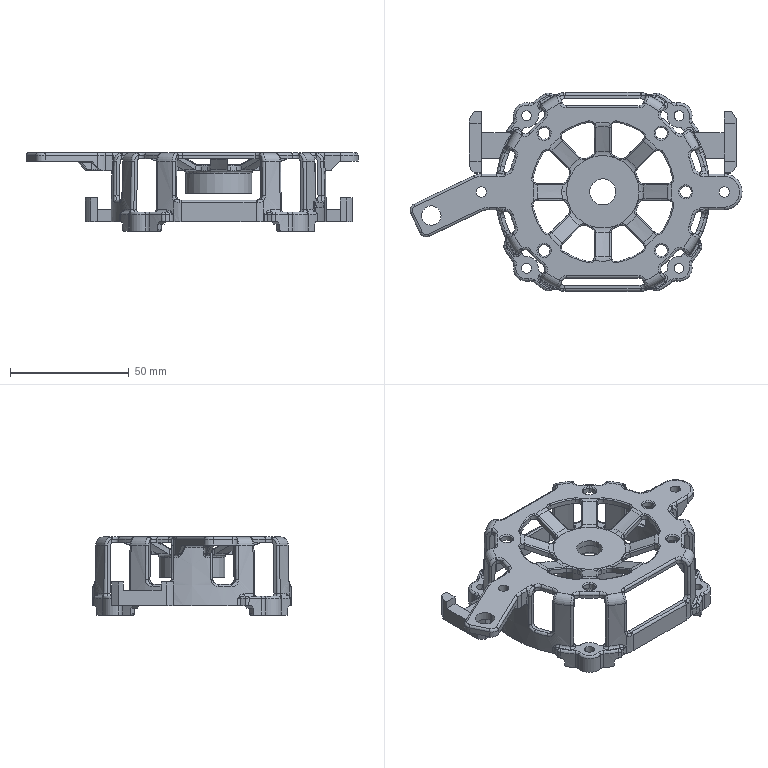Part | STEP file | 1903-QG_1 | 1 solid | 876 faces | box 140.055 x 83.966 x 33 mm | volume 30398 mm3 | cylinder 292 | torus 198 | spline 174 | plane 169 | cone 38 | other 4 | sphere 1 | commonest cylinder face diameters 4 x83 2 x60 1 x41 5 x10 4.2 x8 10 x8